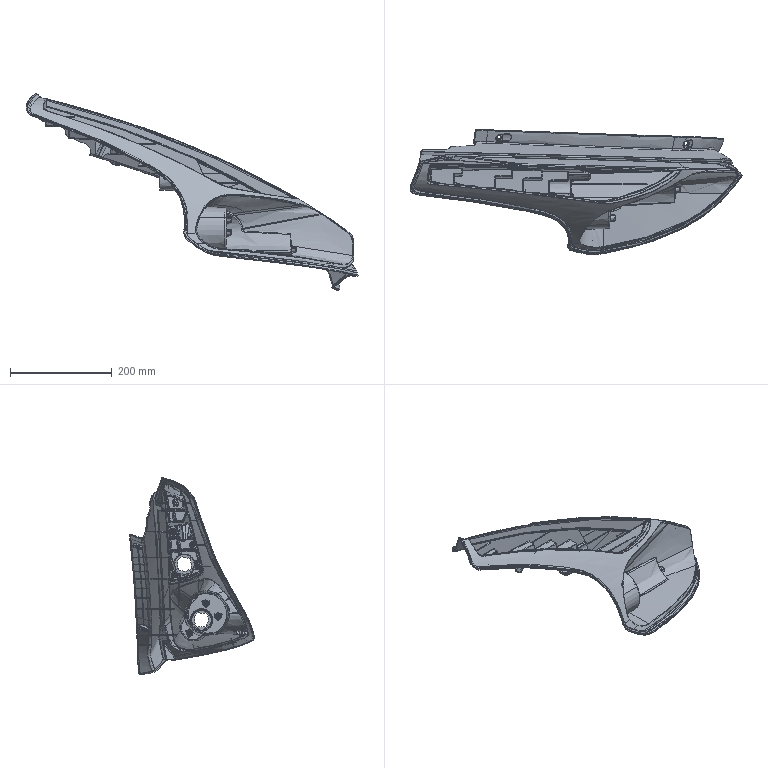Part | STEP file | solid 183 | 1 solid | 1918 faces | box 652.487 x 245.59 x 387.851 mm | volume 667269 mm3 | spline 1416 | plane 227 | sphere 83 | cylinder 78 | cone 58 | torus 46 | other 10 | commonest cylinder face diameters 4.02 x20 2.01 x17 27.135 x8 31.155 x8 2.915 x7 1.005 x6